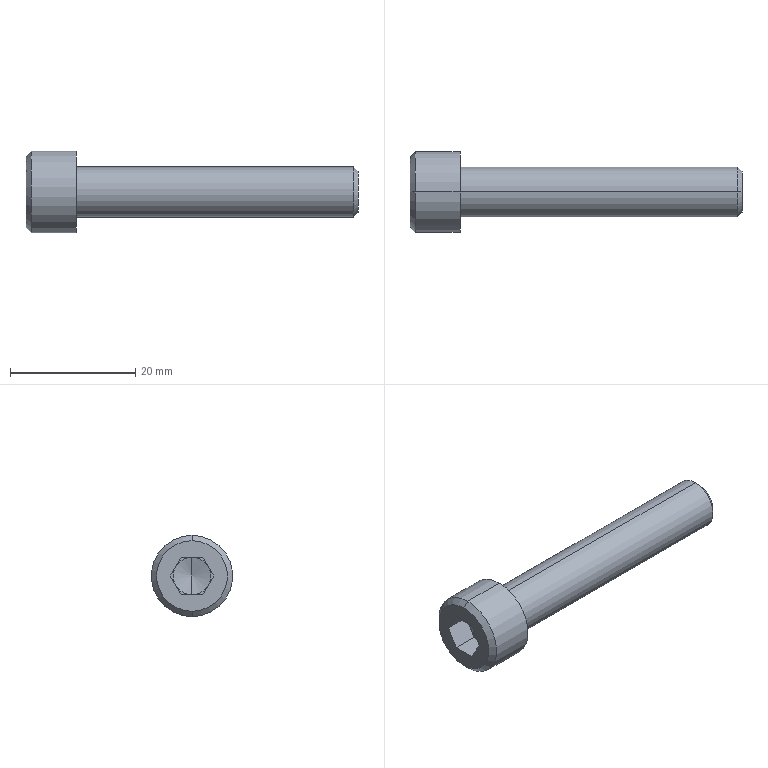Part | STEP file | 0230_304_SCB8-45 | 1 solid | 25 faces | box 53 x 13 x 13 mm | volume 3170 mm3 | plane 15 | cone 6 | cylinder 4 | commonest cylinder face diameters 8 x2 13 x2